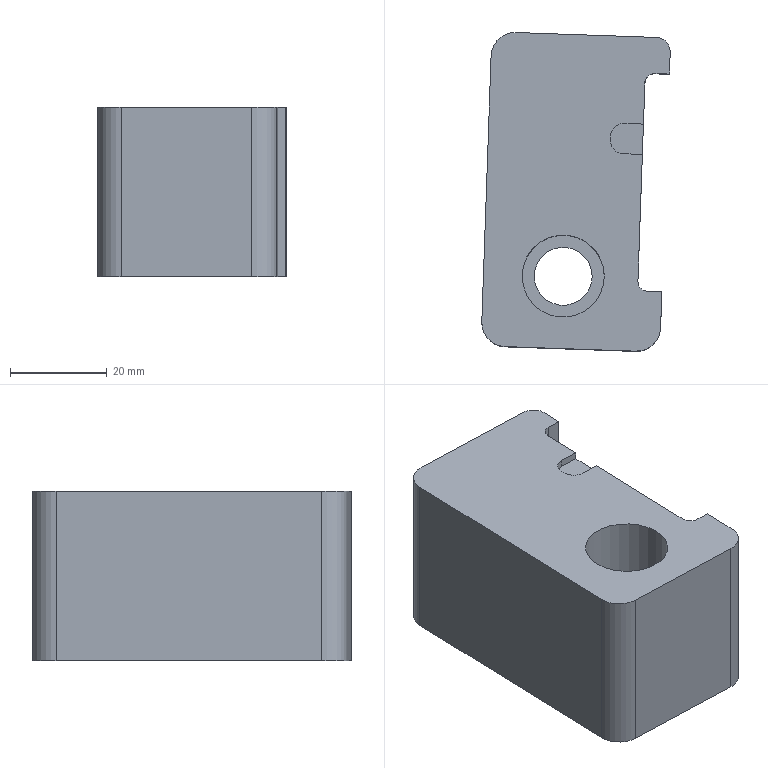Part | NX | features DIE-47 2 | 1 solid | 24 faces | box 38.971 x 65.909 x 35 mm | volume 68711 mm3 | plane 14 | cylinder 8 | spline 2 | commonest cylinder face diameters 10 x3 4.04 x2 6 x1 12.002 x1 17 x1
STEP:
#1=CARTESIAN_POINT('',(2946.663,-896.363,858.716));
#2=VERTEX_POINT('',#1);
#3=CARTESIAN_POINT('',(2946.371,-904.863,858.716));
#4=VERTEX_POINT('',#3);
#5=CARTESIAN_POINT('',(2945.852,-919.349,858.716));
#6=DIRECTION('',(0.0349,0.9994,0.));
#7=VECTOR('',#6,1000.);
#8=LINE('',#5,#7);
#9=EDGE_CURVE('',#2,#4,#8,.F.);
#10=ORIENTED_EDGE('',*,*,#9,.T.);
#11=CARTESIAN_POINT('',(2946.358,-904.862,857.216));
#12=VERTEX_POINT('',#11);
#13=CARTESIAN_POINT('',(2946.358,-904.862,858.716));
#14=DIRECTION('',(0.,0.,-1.));
#15=VECTOR('',#14,1000.);
#16=LINE('',#13,#15);
#17=EDGE_CURVE('',#4,#12,#16,.T.);
#18=ORIENTED_EDGE('',*,*,#17,.T.);
#19=CARTESIAN_POINT('',(2946.139,-911.133,857.216));
#20=VERTEX_POINT('',#19);
#21=CARTESIAN_POINT('',(2946.139,-911.133,857.216));
#22=CARTESIAN_POINT('',(2946.183,-909.878,857.216));
#23=CARTESIAN_POINT('',(2946.226,-908.624,857.216));
#24=CARTESIAN_POINT('',(2946.27,-907.37,857.216));
#25=CARTESIAN_POINT('',(2946.314,-906.116,857.216));
#26=CARTESIAN_POINT('',(2946.358,-904.862,857.216));
#27=B_SPLINE_CURVE_WITH_KNOTS('',5,(#21,#22,#23,#24,#25,#26),.UNSPECIFIED.,.F.,.F.,(6,6),(0.,1.),.PIECEWISE_BEZIER_KNOTS.);
#28=EDGE_CURVE('',#20,#12,#27,.T.);
#29=ORIENTED_EDGE('',*,*,#28,.F.);
#30=CARTESIAN_POINT('',(2946.139,-911.133,858.716));
#31=VERTEX_POINT('',#30);
#32=CARTESIAN_POINT('',(2946.139,-911.133,858.716));
#33=DIRECTION('',(0.,0.,-1.));
#34=VECTOR('',#33,1000.);
#35=LINE('',#32,#34);
#36=EDGE_CURVE('',#20,#31,#35,.F.);
#37=ORIENTED_EDGE('',*,*,#36,.T.);
#38=CARTESIAN_POINT('',(2945.224,-937.338,858.716));
#39=VERTEX_POINT('',#38);
#40=CARTESIAN_POINT('',(2945.852,-919.349,858.716));
#41=DIRECTION('',(0.0349,0.9994,0.));
#42=VECTOR('',#41,1000.);
#43=LINE('',#40,#42);
#44=EDGE_CURVE('',#31,#39,#43,.F.);
#45=ORIENTED_EDGE('',*,*,#44,.T.);
#46=CARTESIAN_POINT('',(2945.224,-937.338,823.716));
#47=VERTEX_POINT('',#46);
#48=CARTESIAN_POINT('',(2945.224,-937.338,858.716));
#49=DIRECTION('',(0.,0.,1.));
#50=VECTOR('',#49,1000.);
#51=LINE('',#48,#50);
#52=EDGE_CURVE('',#39,#47,#51,.F.);
#53=ORIENTED_EDGE('',*,*,#52,.T.);
#54=CARTESIAN_POINT('',(2946.655,-896.363,823.716));
#55=VERTEX_POINT('',#54);
#56=CARTESIAN_POINT('',(2945.852,-919.349,823.716));
#57=DIRECTION('',(0.0349,0.9994,0.));
#58=VECTOR('',#57,1000.);
#59=LINE('',#56,#58);
#60=EDGE_CURVE('',#47,#55,#59,.T.);
#61=ORIENTED_EDGE('',*,*,#60,.T.);
#62=CARTESIAN_POINT('',(2946.655,-896.363,858.716));
#63=DIRECTION('',(0.,0.,1.));
#64=VECTOR('',#63,1000.);
#65=LINE('',#62,#64);
#66=EDGE_CURVE('',#55,#2,#65,.T.);
#67=ORIENTED_EDGE('',*,*,#66,.T.);
#68=EDGE_LOOP('',(#10,#18,#29,#37,#45,#53,#61,#67));
#69=FACE_BOUND('',#68,.T.);
#70=CARTESIAN_POINT('',(2945.852,-919.349,858.716));
#71=DIRECTION('',(0.9994,-0.0349,0.));
#72=DIRECTION('',(0.0349,0.9994,0.));
#73=AXIS2_PLACEMENT_3D('',#70,#71,#72);
#74=PLANE('',#73);
#75=ADVANCED_FACE('',(#69),#74,.T.);
#76=CARTESIAN_POINT('',(2921.271,-936.298,858.716));
#77=VERTEX_POINT('',#76);
#78=CARTESIAN_POINT('',(2929.771,-936.298,858.716));
#79=DIRECTION('',(0.,0.,-1.));
#80=DIRECTION('',(-1.,0.,0.));
#81=AXIS2_PLACEMENT_3D('',#78,#79,#80);
#82=CIRCLE('',#81,8.5);
#83=EDGE_CURVE('',#77,#77,#82,.T.);
#84=ORIENTED_EDGE('',*,*,#83,.T.);
#85=EDGE_LOOP('',(#84));
#86=FACE_BOUND('',#85,.T.);
#87=CARTESIAN_POINT('',(2917.754,-950.887,858.716));
#88=VERTEX_POINT('',#87);
#89=CARTESIAN_POINT('',(2944.738,-951.829,858.716));
#90=VERTEX_POINT('',#89);
#91=CARTESIAN_POINT('',(2936.743,-951.55,858.716));
#92=DIRECTION('',(-0.9994,0.0349,0.));
#93=VECTOR('',#92,1000.);
#94=LINE('',#91,#93);
#95=EDGE_CURVE('',#88,#90,#94,.F.);
#96=ORIENTED_EDGE('',*,*,#95,.T.);
#97=CARTESIAN_POINT('',(2949.909,-947.007,858.716));
#98=VERTEX_POINT('',#97);
#99=CARTESIAN_POINT('',(2944.912,-946.833,858.716));
#100=DIRECTION('',(0.,0.,-1.));
#101=DIRECTION('',(-1.,0.,0.));
#102=AXIS2_PLACEMENT_3D('',#99,#100,#101);
#103=CIRCLE('',#102,5.);
#104=EDGE_CURVE('',#90,#98,#103,.F.);
#105=ORIENTED_EDGE('',*,*,#104,.T.);
#106=CARTESIAN_POINT('',(2950.17,-939.532,858.716));
#107=VERTEX_POINT('',#106);
#108=CARTESIAN_POINT('',(2950.869,-919.524,858.716));
#109=DIRECTION('',(0.0349,0.9994,0.));
#110=VECTOR('',#109,1000.);
#111=LINE('',#108,#110);
#112=EDGE_CURVE('',#107,#98,#111,.F.);
#113=ORIENTED_EDGE('',*,*,#112,.F.);
#114=CARTESIAN_POINT('',(2947.172,-939.427,858.716));
#115=VERTEX_POINT('',#114);
#116=CARTESIAN_POINT('',(2956.52,-939.753,858.716));
#117=DIRECTION('',(0.9994,-0.0349,0.));
#118=VECTOR('',#117,1000.);
#119=LINE('',#116,#118);
#120=EDGE_CURVE('',#107,#115,#119,.F.);
#121=ORIENTED_EDGE('',*,*,#120,.T.);
#122=CARTESIAN_POINT('',(2947.243,-937.408,858.716));
#123=DIRECTION('',(0.,0.,1.));
#124=DIRECTION('',(1.,0.,0.));
#125=AXIS2_PLACEMENT_3D('',#122,#123,#124);
#126=CIRCLE('',#125,2.02);
#127=EDGE_CURVE('',#39,#115,#126,.T.);
#128=ORIENTED_EDGE('',*,*,#127,.F.);
#129=ORIENTED_EDGE('',*,*,#44,.F.);
#130=CARTESIAN_POINT('',(2942.1,-910.991,858.716));
#131=VERTEX_POINT('',#130);
#132=CARTESIAN_POINT('',(2946.139,-911.133,858.716));
#133=CARTESIAN_POINT('',(2944.792,-911.086,858.716));
#134=CARTESIAN_POINT('',(2943.446,-911.039,858.716));
#135=CARTESIAN_POINT('',(2942.1,-910.991,858.716));
#136=B_SPLINE_CURVE_WITH_KNOTS('',3,(#132,#133,#134,#135),.UNSPECIFIED.,.F.,.F.,(4,4),(0.00502,0.009061),.UNSPECIFIED.);
#137=EDGE_CURVE('',#31,#131,#136,.T.);
#138=ORIENTED_EDGE('',*,*,#137,.T.);
#139=CARTESIAN_POINT('',(2940.946,-910.666,858.716));
#140=VERTEX_POINT('',#139);
#141=CARTESIAN_POINT('',(2942.1,-910.991,858.716));
#142=CARTESIAN_POINT('',(2941.681,-910.977,858.716));
#143=CARTESIAN_POINT('',(2941.297,-910.868,858.716));
#144=CARTESIAN_POINT('',(2940.946,-910.666,858.716));
#145=B_SPLINE_CURVE_WITH_KNOTS('',3,(#141,#142,#143,#144),.UNSPECIFIED.,.F.,.F.,(4,4),(0.,1.),.UNSPECIFIED.);
#146=EDGE_CURVE('',#131,#140,#145,.T.);
#147=ORIENTED_EDGE('',*,*,#146,.T.);
#148=CARTESIAN_POINT('',(2940.072,-909.843,858.716));
#149=VERTEX_POINT('',#148);
#150=CARTESIAN_POINT('',(2940.946,-910.666,858.716));
#151=CARTESIAN_POINT('',(2940.6,-910.467,858.716));
#152=CARTESIAN_POINT('',(2940.305,-910.184,858.716));
#153=CARTESIAN_POINT('',(2940.072,-909.843,858.716));
#154=B_SPLINE_CURVE_WITH_KNOTS('',3,(#150,#151,#152,#153),.UNSPECIFIED.,.F.,.F.,(4,4),(0.,1.),.UNSPECIFIED.);
#155=EDGE_CURVE('',#140,#149,#154,.T.);
#156=ORIENTED_EDGE('',*,*,#155,.T.);
#157=CARTESIAN_POINT('',(2939.671,-909.031,858.716));
#158=VERTEX_POINT('',#157);
#159=CARTESIAN_POINT('',(2940.072,-909.843,858.716));
#160=CARTESIAN_POINT('',(2939.904,-909.597,858.716));
#161=CARTESIAN_POINT('',(2939.77,-909.326,858.716));
#162=CARTESIAN_POINT('',(2939.671,-909.031,858.716));
#163=B_SPLINE_CURVE_WITH_KNOTS('',3,(#159,#160,#161,#162),.UNSPECIFIED.,.F.,.F.,(4,4),(0.,1.),.UNSPECIFIED.);
#164=EDGE_CURVE('',#149,#158,#163,.T.);
#165=ORIENTED_EDGE('',*,*,#164,.T.);
#166=CARTESIAN_POINT('',(2939.499,-907.537,858.716));
#167=VERTEX_POINT('',#166);
#168=CARTESIAN_POINT('',(2939.671,-909.031,858.716));
#169=CARTESIAN_POINT('',(2939.59,-908.79,858.716));
#170=CARTESIAN_POINT('',(2939.507,-908.413,858.716));
#171=CARTESIAN_POINT('',(2939.478,-907.989,858.716));
#172=CARTESIAN_POINT('',(2939.484,-907.712,858.716));
#173=CARTESIAN_POINT('',(2939.49,-907.634,858.716));
#174=CARTESIAN_POINT('',(2939.498,-907.537,858.716));
#175=B_SPLINE_CURVE_WITH_KNOTS('',3,(#168,#169,#170,#171,#172,#173,#174),.UNSPECIFIED.,.F.,.F.,(4,1,1,1,4),(0.,0.5,0.75,0.875,1.),.UNSPECIFIED.);
#176=EDGE_CURVE('',#158,#167,#175,.T.);
#177=ORIENTED_EDGE('',*,*,#176,.T.);
#178=CARTESIAN_POINT('',(2940.362,-905.554,858.716));
#179=VERTEX_POINT('',#178);
#180=CARTESIAN_POINT('',(2939.499,-907.537,858.716));
#181=CARTESIAN_POINT('',(2939.573,-906.799,858.716));
#182=CARTESIAN_POINT('',(2939.876,-906.079,858.716));
#183=CARTESIAN_POINT('',(2940.362,-905.554,858.716));
#184=B_SPLINE_CURVE_WITH_KNOTS('',3,(#180,#181,#182,#183),.UNSPECIFIED.,.F.,.F.,(4,4),(0.,1.),.UNSPECIFIED.);
#185=EDGE_CURVE('',#179,#167,#184,.F.);
#186=ORIENTED_EDGE('',*,*,#185,.F.);
#187=CARTESIAN_POINT('',(2941.247,-904.918,858.716));
#188=VERTEX_POINT('',#187);
#189=CARTESIAN_POINT('',(2940.362,-905.554,858.716));
#190=CARTESIAN_POINT('',(2940.616,-905.279,858.716));
#191=CARTESIAN_POINT('',(2940.914,-905.062,858.716));
#192=CARTESIAN_POINT('',(2941.247,-904.918,858.716));
#193=B_SPLINE_CURVE_WITH_KNOTS('',3,(#189,#190,#191,#192),.UNSPECIFIED.,.F.,.F.,(4,4),(0.,1.),.UNSPECIFIED.);
#194=EDGE_CURVE('',#188,#179,#193,.F.);
#195=ORIENTED_EDGE('',*,*,#194,.F.);
#196=CARTESIAN_POINT('',(2942.319,-904.721,858.716));
#197=VERTEX_POINT('',#196);
#198=CARTESIAN_POINT('',(2941.247,-904.918,858.716));
#199=CARTESIAN_POINT('',(2941.583,-904.774,858.716));
#200=CARTESIAN_POINT('',(2941.94,-904.708,858.716));
#201=CARTESIAN_POINT('',(2942.319,-904.721,858.716));
#202=B_SPLINE_CURVE_WITH_KNOTS('',3,(#198,#199,#200,#201),.UNSPECIFIED.,.F.,.F.,(4,4),(0.,1.),.UNSPECIFIED.);
#203=EDGE_CURVE('',#197,#188,#202,.F.);
#204=ORIENTED_EDGE('',*,*,#203,.F.);
#205=CARTESIAN_POINT('',(2942.319,-904.721,858.716));
#206=CARTESIAN_POINT('',(2943.674,-904.768,858.716));
#207=CARTESIAN_POINT('',(2945.029,-904.816,858.716));
#208=CARTESIAN_POINT('',(2946.384,-904.863,858.716));
#209=B_SPLINE_CURVE_WITH_KNOTS('',3,(#205,#206,#207,#208),.UNSPECIFIED.,.F.,.F.,(4,4),(0.,0.004068),.UNSPECIFIED.);
#210=EDGE_CURVE('',#197,#4,#209,.T.);
#211=ORIENTED_EDGE('',*,*,#210,.T.);
#212=ORIENTED_EDGE('',*,*,#9,.F.);
#213=CARTESIAN_POINT('',(2946.676,-896.134,858.716));
#214=VERTEX_POINT('',#213);
#215=CARTESIAN_POINT('',(2946.676,-896.134,858.716));
#216=CARTESIAN_POINT('',(2946.669,-896.21,858.716));
#217=CARTESIAN_POINT('',(2946.662,-896.286,858.716));
#218=CARTESIAN_POINT('',(2946.655,-896.363,858.716));
#219=B_SPLINE_CURVE_WITH_KNOTS('',3,(#215,#216,#217,#218),.UNSPECIFIED.,.F.,.F.,(4,4),(0.,1.),.UNSPECIFIED.);
#220=EDGE_CURVE('',#214,#2,#219,.T.);
#221=ORIENTED_EDGE('',*,*,#220,.F.);
#222=CARTESIAN_POINT('',(2948.744,-894.414,858.716));
#223=VERTEX_POINT('',#222);
#224=CARTESIAN_POINT('',(2948.673,-896.433,858.716));
#225=DIRECTION('',(0.,0.,1.));
#226=DIRECTION('',(1.,0.,0.));
#227=AXIS2_PLACEMENT_3D('',#224,#225,#226);
#228=CIRCLE('',#227,2.02);
#229=EDGE_CURVE('',#223,#214,#228,.T.);
#230=ORIENTED_EDGE('',*,*,#229,.F.);
#231=CARTESIAN_POINT('',(2951.742,-894.519,858.716));
#232=VERTEX_POINT('',#231);
#233=CARTESIAN_POINT('',(2958.092,-894.741,858.716));
#234=DIRECTION('',(0.9994,-0.0349,0.));
#235=VECTOR('',#234,1000.);
#236=LINE('',#233,#235);
#237=EDGE_CURVE('',#232,#223,#236,.F.);
#238=ORIENTED_EDGE('',*,*,#237,.F.);
#239=CARTESIAN_POINT('',(2951.898,-890.042,858.716));
#240=VERTEX_POINT('',#239);
#241=CARTESIAN_POINT('',(2950.869,-919.524,858.716));
#242=DIRECTION('',(0.0349,0.9994,0.));
#243=VECTOR('',#242,1000.);
#244=LINE('',#241,#243);
#245=EDGE_CURVE('',#240,#232,#244,.F.);
#246=ORIENTED_EDGE('',*,*,#245,.F.);
#247=CARTESIAN_POINT('',(2949.005,-886.939,858.716));
#248=VERTEX_POINT('',#247);
#249=CARTESIAN_POINT('',(2948.9,-889.937,858.716));
#250=DIRECTION('',(0.,0.,-1.));
#251=DIRECTION('',(-1.,0.,0.));
#252=AXIS2_PLACEMENT_3D('',#249,#250,#251);
#253=CIRCLE('',#252,3.);
#254=EDGE_CURVE('',#240,#248,#253,.F.);
#255=ORIENTED_EDGE('',*,*,#254,.T.);
#256=CARTESIAN_POINT('',(2920.022,-885.927,858.716));
#257=VERTEX_POINT('',#256);
#258=CARTESIAN_POINT('',(2939.011,-886.59,858.716));
#259=DIRECTION('',(-0.9994,0.0349,0.));
#260=VECTOR('',#259,1000.);
#261=LINE('',#258,#260);
#262=EDGE_CURVE('',#257,#248,#261,.F.);
#263=ORIENTED_EDGE('',*,*,#262,.F.);
#264=CARTESIAN_POINT('',(2914.851,-890.749,858.716));
#265=VERTEX_POINT('',#264);
#266=CARTESIAN_POINT('',(2919.848,-890.924,858.716));
#267=DIRECTION('',(0.,0.,-1.));
#268=DIRECTION('',(-1.,0.,0.));
#269=AXIS2_PLACEMENT_3D('',#266,#267,#268);
#270=CIRCLE('',#269,5.);
#271=EDGE_CURVE('',#257,#265,#270,.F.);
#272=ORIENTED_EDGE('',*,*,#271,.T.);
#273=CARTESIAN_POINT('',(2912.932,-945.716,858.716));
#274=VERTEX_POINT('',#273);
#275=CARTESIAN_POINT('',(2914.328,-905.74,858.716));
#276=DIRECTION('',(-0.0349,-0.9994,0.));
#277=VECTOR('',#276,1000.);
#278=LINE('',#275,#277);
#279=EDGE_CURVE('',#265,#274,#278,.T.);
#280=ORIENTED_EDGE('',*,*,#279,.T.);
#281=CARTESIAN_POINT('',(2917.929,-945.89,858.716));
#282=DIRECTION('',(0.,0.,-1.));
#283=DIRECTION('',(-1.,0.,0.));
#284=AXIS2_PLACEMENT_3D('',#281,#282,#283);
#285=CIRCLE('',#284,5.);
#286=EDGE_CURVE('',#274,#88,#285,.F.);
#287=ORIENTED_EDGE('',*,*,#286,.T.);
#288=EDGE_LOOP('',(#96,#105,#113,#121,#128,#129,#138,#147,#156,#165,#177,#186,#195,#204,#211,#212,#221,#230,#238,#246,#255,#263,#272,#280,#287));
#289=FACE_BOUND('',#288,.T.);
#290=CARTESIAN_POINT('',(2958.707,-877.122,858.716));
#291=DIRECTION('',(0.,0.,-1.));
#292=DIRECTION('',(0.,1.,0.));
#293=AXIS2_PLACEMENT_3D('',#290,#291,#292);
#294=PLANE('',#293);
#295=ADVANCED_FACE('',(#86,#289),#294,.F.);
#296=CARTESIAN_POINT('',(2951.742,-894.519,823.716));
#297=VERTEX_POINT('',#296);
#298=CARTESIAN_POINT('',(2951.742,-894.519,858.716));
#299=DIRECTION('',(0.,0.,1.));
#300=VECTOR('',#299,1000.);
#301=LINE('',#298,#300);
#302=EDGE_CURVE('',#232,#297,#301,.F.);
#303=ORIENTED_EDGE('',*,*,#302,.T.);
#304=CARTESIAN_POINT('',(2951.898,-890.042,823.716));
#305=VERTEX_POINT('',#304);
#306=CARTESIAN_POINT('',(2950.869,-919.524,823.716));
#307=DIRECTION('',(0.0349,0.9994,0.));
#308=VECTOR('',#307,1000.);
#309=LINE('',#306,#308);
#310=EDGE_CURVE('',#305,#297,#309,.F.);
#311=ORIENTED_EDGE('',*,*,#310,.F.);
#312=CARTESIAN_POINT('',(2951.898,-890.042,858.716));
#313=DIRECTION('',(0.,0.,1.));
#314=VECTOR('',#313,1000.);
#315=LINE('',#312,#314);
#316=EDGE_CURVE('',#305,#240,#315,.T.);
#317=ORIENTED_EDGE('',*,*,#316,.T.);
#318=ORIENTED_EDGE('',*,*,#245,.T.);
#319=EDGE_LOOP('',(#303,#311,#317,#318));
#320=FACE_BOUND('',#319,.T.);
#321=CARTESIAN_POINT('',(2950.869,-919.524,858.716));
#322=DIRECTION('',(0.9994,-0.0349,0.));
#323=DIRECTION('',(0.0349,0.9994,0.));
#324=AXIS2_PLACEMENT_3D('',#321,#322,#323);
#325=PLANE('',#324);
#326=ADVANCED_FACE('',(#320),#325,.T.);
#327=CARTESIAN_POINT('',(2917.754,-950.887,823.716));
#328=VERTEX_POINT('',#327);
#329=CARTESIAN_POINT('',(2912.932,-945.716,823.716));
#330=VERTEX_POINT('',#329);
#331=CARTESIAN_POINT('',(2917.929,-945.89,823.716));
#332=DIRECTION('',(0.,0.,-1.));
#333=DIRECTION('',(-1.,0.,0.));
#334=AXIS2_PLACEMENT_3D('',#331,#332,#333);
#335=CIRCLE('',#334,5.);
#336=EDGE_CURVE('',#328,#330,#335,.T.);
#337=ORIENTED_EDGE('',*,*,#336,.F.);
#338=CARTESIAN_POINT('',(2917.754,-950.887,935.716));
#339=DIRECTION('',(0.,0.,-1.));
#340=VECTOR('',#339,1000.);
#341=LINE('',#338,#340);
#342=EDGE_CURVE('',#88,#328,#341,.T.);
#343=ORIENTED_EDGE('',*,*,#342,.F.);
#344=ORIENTED_EDGE('',*,*,#286,.F.);
#345=CARTESIAN_POINT('',(2912.932,-945.716,898.213));
#346=DIRECTION('',(0.,0.,1.));
#347=VECTOR('',#346,1000.);
#348=LINE('',#345,#347);
#349=EDGE_CURVE('',#330,#274,#348,.T.);
#350=ORIENTED_EDGE('',*,*,#349,.F.);
#351=EDGE_LOOP('',(#337,#343,#344,#350));
#352=FACE_BOUND('',#351,.T.);
#353=CARTESIAN_POINT('',(2917.929,-945.89,935.716));
#354=DIRECTION('',(0.,0.,1.));
#355=DIRECTION('',(1.,0.,0.));
#356=AXIS2_PLACEMENT_3D('',#353,#354,#355);
#357=CYLINDRICAL_SURFACE('',#356,5.);
#358=ADVANCED_FACE('',(#352),#357,.T.);
#359=ORIENTED_EDGE('',*,*,#279,.F.);
#360=CARTESIAN_POINT('',(2914.851,-890.749,823.716));
#361=VERTEX_POINT('',#360);
#362=CARTESIAN_POINT('',(2914.851,-890.749,898.213));
#363=DIRECTION('',(0.,0.,1.));
#364=VECTOR('',#363,1000.);
#365=LINE('',#362,#364);
#366=EDGE_CURVE('',#265,#361,#365,.F.);
#367=ORIENTED_EDGE('',*,*,#366,.T.);
#368=CARTESIAN_POINT('',(2914.358,-904.859,823.716));
#369=DIRECTION('',(0.0349,0.9994,0.));
#370=VECTOR('',#369,1000.);
#371=LINE('',#368,#370);
#372=EDGE_CURVE('',#330,#361,#371,.T.);
#373=ORIENTED_EDGE('',*,*,#372,.F.);
#374=ORIENTED_EDGE('',*,*,#349,.T.);
#375=EDGE_LOOP('',(#359,#367,#373,#374));
#376=FACE_BOUND('',#375,.T.);
#377=CARTESIAN_POINT('',(2914.328,-905.74,898.213));
#378=DIRECTION('',(-0.9994,0.0349,0.));
#379=DIRECTION('',(-0.0349,-0.9994,0.));
#380=AXIS2_PLACEMENT_3D('',#377,#378,#379);
#381=PLANE('',#380);
#382=ADVANCED_FACE('',(#376),#381,.T.);
#383=CARTESIAN_POINT('',(2920.022,-885.927,823.716));
#384=VERTEX_POINT('',#383);
#385=CARTESIAN_POINT('',(2919.848,-890.924,823.716));
#386=DIRECTION('',(0.,0.,-1.));
#387=DIRECTION('',(-1.,0.,0.));
#388=AXIS2_PLACEMENT_3D('',#385,#386,#387);
#389=CIRCLE('',#388,5.);
#390=EDGE_CURVE('',#361,#384,#389,.T.);
#391=ORIENTED_EDGE('',*,*,#390,.F.);
#392=ORIENTED_EDGE('',*,*,#366,.F.);
#393=ORIENTED_EDGE('',*,*,#271,.F.);
#394=CARTESIAN_POINT('',(2920.022,-885.927,898.213));
#395=DIRECTION('',(0.,0.,-1.));
#396=VECTOR('',#395,1000.);
#397=LINE('',#394,#396);
#398=EDGE_CURVE('',#384,#257,#397,.F.);
#399=ORIENTED_EDGE('',*,*,#398,.F.);
#400=EDGE_LOOP('',(#391,#392,#393,#399));
#401=FACE_BOUND('',#400,.T.);
#402=CARTESIAN_POINT('',(2919.848,-890.924,898.213));
#403=DIRECTION('',(0.,0.,-1.));
#404=DIRECTION('',(-1.,0.,0.));
#405=AXIS2_PLACEMENT_3D('',#402,#403,#404);
#406=CYLINDRICAL_SURFACE('',#405,5.);
#407=ADVANCED_FACE('',(#401),#406,.T.);
#408=CARTESIAN_POINT('',(2944.738,-951.829,823.716));
#409=VERTEX_POINT('',#408);
#410=CARTESIAN_POINT('',(2965.665,-952.56,823.716));
#411=DIRECTION('',(0.9994,-0.0349,0.));
#412=VECTOR('',#411,1000.);
#413=LINE('',#410,#412);
#414=EDGE_CURVE('',#409,#328,#413,.F.);
#415=ORIENTED_EDGE('',*,*,#414,.F.);
#416=CARTESIAN_POINT('',(2944.738,-951.829,935.716));
#417=DIRECTION('',(0.,0.,1.));
#418=VECTOR('',#417,1000.);
#419=LINE('',#416,#418);
#420=EDGE_CURVE('',#409,#90,#419,.T.);
#421=ORIENTED_EDGE('',*,*,#420,.T.);
#422=ORIENTED_EDGE('',*,*,#95,.F.);
#423=ORIENTED_EDGE('',*,*,#342,.T.);
#424=EDGE_LOOP('',(#415,#421,#422,#423));
#425=FACE_BOUND('',#424,.T.);
#426=CARTESIAN_POINT('',(2936.743,-951.55,935.716));
#427=DIRECTION('',(0.0349,0.9994,0.));
#428=DIRECTION('',(-0.9994,0.0349,0.));
#429=AXIS2_PLACEMENT_3D('',#426,#427,#428);
#430=PLANE('',#429);
#431=ADVANCED_FACE('',(#425),#430,.F.);
#432=ORIENTED_EDGE('',*,*,#262,.T.);
#433=CARTESIAN_POINT('',(2949.005,-886.939,823.716));
#434=VERTEX_POINT('',#433);
#435=CARTESIAN_POINT('',(2949.005,-886.939,823.716));
#436=DIRECTION('',(0.,0.,-1.));
#437=VECTOR('',#436,1000.);
#438=LINE('',#435,#437);
#439=EDGE_CURVE('',#248,#434,#438,.T.);
#440=ORIENTED_EDGE('',*,*,#439,.T.);
#441=CARTESIAN_POINT('',(2967.933,-887.6,823.716));
#442=DIRECTION('',(0.9994,-0.0349,0.));
#443=VECTOR('',#442,1000.);
#444=LINE('',#441,#443);
#445=EDGE_CURVE('',#434,#384,#444,.F.);
#446=ORIENTED_EDGE('',*,*,#445,.T.);
#447=ORIENTED_EDGE('',*,*,#398,.T.);
#448=EDGE_LOOP('',(#432,#440,#446,#447));
#449=FACE_BOUND('',#448,.T.);
#450=CARTESIAN_POINT('',(2939.011,-886.59,935.716));
#451=DIRECTION('',(0.0349,0.9994,0.));
#452=DIRECTION('',(-0.9994,0.0349,0.));
#453=AXIS2_PLACEMENT_3D('',#450,#451,#452);
#454=PLANE('',#453);
#455=ADVANCED_FACE('',(#449),#454,.T.);
#456=CARTESIAN_POINT('',(2923.77,-936.298,823.716));
#457=VERTEX_POINT('',#456);
#458=CARTESIAN_POINT('',(2929.771,-936.298,823.716));
#459=DIRECTION('',(0.,0.,-1.));
#460=DIRECTION('',(-1.,0.,0.));
#461=AXIS2_PLACEMENT_3D('',#458,#459,#460);
#462=CIRCLE('',#461,6.001);
#463=EDGE_CURVE('',#457,#457,#462,.T.);
#464=ORIENTED_EDGE('',*,*,#463,.F.);
#465=EDGE_LOOP('',(#464));
#466=FACE_BOUND('',#465,.T.);
#467=CARTESIAN_POINT('',(2950.17,-939.532,823.716));
#468=VERTEX_POINT('',#467);
#469=CARTESIAN_POINT('',(2949.909,-947.007,823.716));
#470=VERTEX_POINT('',#469);
#471=CARTESIAN_POINT('',(2950.869,-919.524,823.716));
#472=DIRECTION('',(0.0349,0.9994,0.));
#473=VECTOR('',#472,1000.);
#474=LINE('',#471,#473);
#475=EDGE_CURVE('',#468,#470,#474,.F.);
#476=ORIENTED_EDGE('',*,*,#475,.T.);
#477=CARTESIAN_POINT('',(2944.912,-946.833,823.716));
#478=DIRECTION('',(0.,0.,-1.));
#479=DIRECTION('',(-1.,0.,0.));
#480=AXIS2_PLACEMENT_3D('',#477,#478,#479);
#481=CIRCLE('',#480,5.);
#482=EDGE_CURVE('',#470,#409,#481,.T.);
#483=ORIENTED_EDGE('',*,*,#482,.T.);
#484=ORIENTED_EDGE('',*,*,#414,.T.);
#485=ORIENTED_EDGE('',*,*,#336,.T.);
#486=ORIENTED_EDGE('',*,*,#372,.T.);
#487=ORIENTED_EDGE('',*,*,#390,.T.);
#488=ORIENTED_EDGE('',*,*,#445,.F.);
#489=CARTESIAN_POINT('',(2948.9,-889.937,823.716));
#490=DIRECTION('',(0.,0.,-1.));
#491=DIRECTION('',(-1.,0.,0.));
#492=AXIS2_PLACEMENT_3D('',#489,#490,#491);
#493=CIRCLE('',#492,3.);
#494=EDGE_CURVE('',#434,#305,#493,.T.);
#495=ORIENTED_EDGE('',*,*,#494,.T.);
#496=ORIENTED_EDGE('',*,*,#310,.T.);
#497=CARTESIAN_POINT('',(2948.744,-894.414,823.716));
#498=VERTEX_POINT('',#497);
#499=CARTESIAN_POINT('',(2967.672,-895.075,823.716));
#500=DIRECTION('',(0.9994,-0.0349,0.));
#501=VECTOR('',#500,1000.);
#502=LINE('',#499,#501);
#503=EDGE_CURVE('',#297,#498,#502,.F.);
#504=ORIENTED_EDGE('',*,*,#503,.T.);
#505=CARTESIAN_POINT('',(2948.673,-896.433,823.716));
#506=DIRECTION('',(0.,0.,1.));
#507=DIRECTION('',(1.,0.,0.));
#508=AXIS2_PLACEMENT_3D('',#505,#506,#507);
#509=CIRCLE('',#508,2.02);
#510=EDGE_CURVE('',#55,#498,#509,.F.);
#511=ORIENTED_EDGE('',*,*,#510,.F.);
#512=ORIENTED_EDGE('',*,*,#60,.F.);
#513=CARTESIAN_POINT('',(2947.172,-939.427,823.716));
#514=VERTEX_POINT('',#513);
#515=CARTESIAN_POINT('',(2947.243,-937.408,823.716));
#516=DIRECTION('',(0.,0.,1.));
#517=DIRECTION('',(1.,0.,0.));
#518=AXIS2_PLACEMENT_3D('',#515,#516,#517);
#519=CIRCLE('',#518,2.02);
#520=EDGE_CURVE('',#47,#514,#519,.T.);
#521=ORIENTED_EDGE('',*,*,#520,.T.);
#522=CARTESIAN_POINT('',(2966.1,-940.088,823.716));
#523=DIRECTION('',(0.9994,-0.0349,0.));
#524=VECTOR('',#523,1000.);
#525=LINE('',#522,#524);
#526=EDGE_CURVE('',#514,#468,#525,.T.);
#527=ORIENTED_EDGE('',*,*,#526,.T.);
#528=EDGE_LOOP('',(#476,#483,#484,#485,#486,#487,#488,#495,#496,#504,#511,#512,#521,#527));
#529=FACE_BOUND('',#528,.T.);
#530=CARTESIAN_POINT('',(2967.266,-906.707,823.716));
#531=DIRECTION('',(0.,0.,-1.));
#532=DIRECTION('',(0.0349,0.9994,0.));
#533=AXIS2_PLACEMENT_3D('',#530,#531,#532);
#534=PLANE('',#533);
#535=ADVANCED_FACE('',(#466,#529),#534,.T.);
#536=ORIENTED_EDGE('',*,*,#112,.T.);
#537=CARTESIAN_POINT('',(2949.909,-947.007,858.716));
#538=DIRECTION('',(0.,0.,-1.));
#539=VECTOR('',#538,1000.);
#540=LINE('',#537,#539);
#541=EDGE_CURVE('',#98,#470,#540,.T.);
#542=ORIENTED_EDGE('',*,*,#541,.T.);
#543=ORIENTED_EDGE('',*,*,#475,.F.);
#544=CARTESIAN_POINT('',(2950.17,-939.532,858.716));
#545=DIRECTION('',(0.,0.,1.));
#546=VECTOR('',#545,1000.);
#547=LINE('',#544,#546);
#548=EDGE_CURVE('',#468,#107,#547,.T.);
#549=ORIENTED_EDGE('',*,*,#548,.T.);
#550=EDGE_LOOP('',(#536,#542,#543,#549));
#551=FACE_BOUND('',#550,.T.);
#552=CARTESIAN_POINT('',(2950.869,-919.524,858.716));
#553=DIRECTION('',(0.9994,-0.0349,0.));
#554=DIRECTION('',(0.0349,0.9994,0.));
#555=AXIS2_PLACEMENT_3D('',#552,#553,#554);
#556=PLANE('',#555);
#557=ADVANCED_FACE('',(#551),#556,.T.);
#558=ORIENTED_EDGE('',*,*,#254,.F.);
#559=ORIENTED_EDGE('',*,*,#316,.F.);
#560=ORIENTED_EDGE('',*,*,#494,.F.);
#561=ORIENTED_EDGE('',*,*,#439,.F.);
#562=EDGE_LOOP('',(#558,#559,#560,#561));
#563=FACE_BOUND('',#562,.T.);
#564=CARTESIAN_POINT('',(2948.9,-889.937,935.716));
#565=DIRECTION('',(0.,0.,-1.));
#566=DIRECTION('',(-1.,0.,0.));
#567=AXIS2_PLACEMENT_3D('',#564,#565,#566);
#568=CYLINDRICAL_SURFACE('',#567,3.);
#569=ADVANCED_FACE('',(#563),#568,.T.);
#570=ORIENTED_EDGE('',*,*,#237,.T.);
#571=CARTESIAN_POINT('',(2948.744,-894.414,858.716));
#572=DIRECTION('',(0.,0.,1.));
#573=VECTOR('',#572,1000.);
#574=LINE('',#571,#573);
#575=EDGE_CURVE('',#223,#498,#574,.F.);
#576=ORIENTED_EDGE('',*,*,#575,.T.);
#577=ORIENTED_EDGE('',*,*,#503,.F.);
#578=ORIENTED_EDGE('',*,*,#302,.F.);
#579=EDGE_LOOP('',(#570,#576,#577,#578));
#580=FACE_BOUND('',#579,.T.);
#581=CARTESIAN_POINT('',(2938.75,-894.065,935.716));
#582=DIRECTION('',(0.0349,0.9994,0.));
#583=DIRECTION('',(-0.9994,0.0349,0.));
#584=AXIS2_PLACEMENT_3D('',#581,#582,#583);
#585=PLANE('',#584);
#586=ADVANCED_FACE('',(#580),#585,.F.);
#587=ORIENTED_EDGE('',*,*,#220,.T.);
#588=ORIENTED_EDGE('',*,*,#66,.F.);
#589=ORIENTED_EDGE('',*,*,#510,.T.);
#590=ORIENTED_EDGE('',*,*,#575,.F.);
#591=ORIENTED_EDGE('',*,*,#229,.T.);
#592=EDGE_LOOP('',(#587,#588,#589,#590,#591));
#593=FACE_BOUND('',#592,.T.);
#594=CARTESIAN_POINT('',(2948.673,-896.433,858.716));
#595=DIRECTION('',(0.,0.,1.));
#596=DIRECTION('',(1.,0.,0.));
#597=AXIS2_PLACEMENT_3D('',#594,#595,#596);
#598=CYLINDRICAL_SURFACE('',#597,2.02);
#599=ADVANCED_FACE('',(#593),#598,.F.);
#600=CARTESIAN_POINT('',(2947.172,-939.427,858.716));
#601=DIRECTION('',(0.,0.,1.));
#602=VECTOR('',#601,1000.);
#603=LINE('',#600,#602);
#604=EDGE_CURVE('',#514,#115,#603,.T.);
#605=ORIENTED_EDGE('',*,*,#604,.F.);
#606=ORIENTED_EDGE('',*,*,#520,.F.);
#607=ORIENTED_EDGE('',*,*,#52,.F.);
#608=ORIENTED_EDGE('',*,*,#127,.T.);
#609=EDGE_LOOP('',(#605,#606,#607,#608));
#610=FACE_BOUND('',#609,.T.);
#611=CARTESIAN_POINT('',(2947.243,-937.408,858.716));
#612=DIRECTION('',(0.,0.,1.));
#613=DIRECTION('',(1.,0.,0.));
#614=AXIS2_PLACEMENT_3D('',#611,#612,#613);
#615=CYLINDRICAL_SURFACE('',#614,2.02);
#616=ADVANCED_FACE('',(#610),#615,.F.);
#617=ORIENTED_EDGE('',*,*,#548,.F.);
#618=ORIENTED_EDGE('',*,*,#526,.F.);
#619=ORIENTED_EDGE('',*,*,#604,.T.);
#620=ORIENTED_EDGE('',*,*,#120,.F.);
#621=EDGE_LOOP('',(#617,#618,#619,#620));
#622=FACE_BOUND('',#621,.T.);
#623=CARTESIAN_POINT('',(2937.178,-939.078,935.716));
#624=DIRECTION('',(0.0349,0.9994,0.));
#625=DIRECTION('',(-0.9994,0.0349,0.));
#626=AXIS2_PLACEMENT_3D('',#623,#624,#625);
#627=PLANE('',#626);
#628=ADVANCED_FACE('',(#622),#627,.T.);
#629=CARTESIAN_POINT('',(2921.271,-936.298,832.716));
#630=VERTEX_POINT('',#629);
#631=CARTESIAN_POINT('',(2929.771,-936.298,832.716));
#632=DIRECTION('',(0.,0.,-1.));
#633=DIRECTION('',(-1.,0.,0.));
#634=AXIS2_PLACEMENT_3D('',#631,#632,#633);
#635=CIRCLE('',#634,8.5);
#636=EDGE_CURVE('',#630,#630,#635,.T.);
#637=ORIENTED_EDGE('',*,*,#636,.T.);
#638=EDGE_LOOP('',(#637));
#639=FACE_BOUND('',#638,.T.);
#640=ORIENTED_EDGE('',*,*,#83,.F.);
#641=EDGE_LOOP('',(#640));
#642=FACE_BOUND('',#641,.T.);
#643=CARTESIAN_POINT('',(2929.771,-936.298,843.716));
#644=DIRECTION('',(0.,0.,1.));
#645=DIRECTION('',(1.,0.,0.));
#646=AXIS2_PLACEMENT_3D('',#643,#644,#645);
#647=CYLINDRICAL_SURFACE('',#646,8.5);
#648=ADVANCED_FACE('',(#639,#642),#647,.F.);
#649=ORIENTED_EDGE('',*,*,#463,.T.);
#650=EDGE_LOOP('',(#649));
#651=FACE_BOUND('',#650,.T.);
#652=CARTESIAN_POINT('',(2923.77,-936.298,832.716));
#653=VERTEX_POINT('',#652);
#654=CARTESIAN_POINT('',(2929.771,-936.298,832.716));
#655=DIRECTION('',(0.,0.,-1.));
#656=DIRECTION('',(-1.,0.,0.));
#657=AXIS2_PLACEMENT_3D('',#654,#655,#656);
#658=CIRCLE('',#657,6.001);
#659=EDGE_CURVE('',#653,#653,#658,.T.);
#660=ORIENTED_EDGE('',*,*,#659,.F.);
#661=EDGE_LOOP('',(#660));
#662=FACE_BOUND('',#661,.T.);
#663=CARTESIAN_POINT('',(2929.771,-936.298,808.716));
#664=DIRECTION('',(0.,0.,1.));
#665=DIRECTION('',(1.,0.,0.));
#666=AXIS2_PLACEMENT_3D('',#663,#664,#665);
#667=CYLINDRICAL_SURFACE('',#666,6.001);
#668=ADVANCED_FACE('',(#651,#662),#667,.F.);
#669=ORIENTED_EDGE('',*,*,#659,.T.);
#670=EDGE_LOOP('',(#669));
#671=FACE_BOUND('',#670,.T.);
#672=ORIENTED_EDGE('',*,*,#636,.F.);
#673=EDGE_LOOP('',(#672));
#674=FACE_BOUND('',#673,.T.);
#675=CARTESIAN_POINT('',(2929.771,-936.298,832.716));
#676=DIRECTION('',(0.,0.,-1.));
#677=DIRECTION('',(-1.,0.,0.));
#678=AXIS2_PLACEMENT_3D('',#675,#676,#677);
#679=PLANE('',#678);
#680=ADVANCED_FACE('',(#671,#674),#679,.F.);
#681=ORIENTED_EDGE('',*,*,#482,.F.);
#682=ORIENTED_EDGE('',*,*,#541,.F.);
#683=ORIENTED_EDGE('',*,*,#104,.F.);
#684=ORIENTED_EDGE('',*,*,#420,.F.);
#685=EDGE_LOOP('',(#681,#682,#683,#684));
#686=FACE_BOUND('',#685,.T.);
#687=CARTESIAN_POINT('',(2944.912,-946.833,935.716));
#688=DIRECTION('',(0.,0.,-1.));
#689=DIRECTION('',(-1.,0.,0.));
#690=AXIS2_PLACEMENT_3D('',#687,#688,#689);
#691=CYLINDRICAL_SURFACE('',#690,5.);
#692=ADVANCED_FACE('',(#686),#691,.T.);
#693=ORIENTED_EDGE('',*,*,#28,.T.);
#694=CARTESIAN_POINT('',(2942.319,-904.721,857.216));
#695=VERTEX_POINT('',#694);
#696=CARTESIAN_POINT('',(2942.319,-904.721,857.216));
#697=CARTESIAN_POINT('',(2942.493,-904.727,857.216));
#698=CARTESIAN_POINT('',(2942.668,-904.733,857.216));
#699=CARTESIAN_POINT('',(2942.843,-904.739,857.216));
#700=CARTESIAN_POINT('',(2943.842,-904.774,857.216));
#701=CARTESIAN_POINT('',(2944.841,-904.809,857.216));
#702=CARTESIAN_POINT('',(2945.841,-904.844,857.216));
#703=CARTESIAN_POINT('',(2946.022,-904.85,857.216));
#704=CARTESIAN_POINT('',(2946.203,-904.857,857.216));
#705=CARTESIAN_POINT('',(2946.384,-904.863,857.216));
#706=B_SPLINE_CURVE_WITH_KNOTS('',3,(#696,#697,#698,#699,#700,#701,#702,#703,#704,#705),.UNSPECIFIED.,.F.,.F.,(4,3,3,4),(0.,0.1289,0.8664,1.),.PIECEWISE_BEZIER_KNOTS.);
#707=EDGE_CURVE('',#695,#12,#706,.T.);
#708=ORIENTED_EDGE('',*,*,#707,.F.);
#709=CARTESIAN_POINT('',(2939.499,-907.537,857.216));
#710=VERTEX_POINT('',#709);
#711=CARTESIAN_POINT('',(2939.499,-907.537,857.216));
#712=CARTESIAN_POINT('',(2939.573,-906.803,857.216));
#713=CARTESIAN_POINT('',(2939.866,-906.09,857.216));
#714=CARTESIAN_POINT('',(2940.61,-905.285,857.216));
#715=CARTESIAN_POINT('',(2940.912,-905.063,857.216));
#716=CARTESIAN_POINT('',(2941.583,-904.774,857.216));
#717=CARTESIAN_POINT('',(2941.95,-904.708,857.216));
#718=CARTESIAN_POINT('',(2942.319,-904.721,857.216));
#719=B_SPLINE_CURVE_WITH_KNOTS('',3,(#711,#712,#713,#714,#715,#716,#717,#718),.UNSPECIFIED.,.F.,.F.,(4,2,2,4),(0.,0.5,0.75,1.),.UNSPECIFIED.);
#720=EDGE_CURVE('',#710,#695,#719,.T.);
#721=ORIENTED_EDGE('',*,*,#720,.F.);
#722=CARTESIAN_POINT('',(2942.1,-910.991,857.216));
#723=VERTEX_POINT('',#722);
#724=CARTESIAN_POINT('',(2942.1,-910.991,857.216));
#725=CARTESIAN_POINT('',(2941.693,-910.977,857.216));
#726=CARTESIAN_POINT('',(2941.294,-910.867,857.216));
#727=CARTESIAN_POINT('',(2940.598,-910.465,857.216));
#728=CARTESIAN_POINT('',(2940.3,-910.177,857.216));
#729=CARTESIAN_POINT('',(2939.843,-909.508,857.216));
#730=CARTESIAN_POINT('',(2939.682,-909.131,857.216));
#731=CARTESIAN_POINT('',(2939.489,-908.345,857.216));
#732=CARTESIAN_POINT('',(2939.464,-907.942,857.216));
#733=CARTESIAN_POINT('',(2939.498,-907.537,857.216));
#734=B_SPLINE_CURVE_WITH_KNOTS('',3,(#724,#725,#726,#727,#728,#729,#730,#731,#732,#733),.UNSPECIFIED.,.F.,.F.,(4,2,2,2,4),(0.,0.25,0.5,0.75,1.),.UNSPECIFIED.);
#735=EDGE_CURVE('',#723,#710,#734,.T.);
#736=ORIENTED_EDGE('',*,*,#735,.F.);
#737=CARTESIAN_POINT('',(2946.139,-911.133,857.216));
#738=CARTESIAN_POINT('',(2944.792,-911.086,857.216));
#739=CARTESIAN_POINT('',(2943.446,-911.039,857.216));
#740=CARTESIAN_POINT('',(2942.1,-910.991,857.216));
#741=B_SPLINE_CURVE_WITH_KNOTS('',3,(#737,#738,#739,#740),.UNSPECIFIED.,.F.,.F.,(4,4),(0.,1.),.PIECEWISE_BEZIER_KNOTS.);
#742=EDGE_CURVE('',#20,#723,#741,.T.);
#743=ORIENTED_EDGE('',*,*,#742,.F.);
#744=EDGE_LOOP('',(#693,#708,#721,#736,#743));
#745=FACE_BOUND('',#744,.T.);
#746=CARTESIAN_POINT('',(2939.498,-907.537,857.216));
#747=DIRECTION('',(0.,0.,1.));
#748=DIRECTION('',(0.,-1.,0.));
#749=AXIS2_PLACEMENT_3D('',#746,#747,#748);
#750=PLANE('',#749);
#751=ADVANCED_FACE('',(#745),#750,.T.);
#752=ORIENTED_EDGE('',*,*,#720,.T.);
#753=CARTESIAN_POINT('',(2942.319,-904.721,858.716));
#754=DIRECTION('',(0.,0.,-1.));
#755=VECTOR('',#754,1000.);
#756=LINE('',#753,#755);
#757=EDGE_CURVE('',#197,#695,#756,.T.);
#758=ORIENTED_EDGE('',*,*,#757,.F.);
#759=ORIENTED_EDGE('',*,*,#203,.T.);
#760=ORIENTED_EDGE('',*,*,#194,.T.);
#761=ORIENTED_EDGE('',*,*,#185,.T.);
#762=CARTESIAN_POINT('',(2939.499,-907.537,857.216));
#763=CARTESIAN_POINT('',(2939.499,-907.537,857.716));
#764=CARTESIAN_POINT('',(2939.499,-907.537,858.216));
#765=CARTESIAN_POINT('',(2939.499,-907.537,858.716));
#766=B_SPLINE_CURVE_WITH_KNOTS('',3,(#762,#763,#764,#765),.UNSPECIFIED.,.F.,.F.,(4,4),(0.,1.),.UNSPECIFIED.);
#767=EDGE_CURVE('',#167,#710,#766,.F.);
#768=ORIENTED_EDGE('',*,*,#767,.T.);
#769=EDGE_LOOP('',(#752,#758,#759,#760,#761,#768));
#770=FACE_BOUND('',#769,.T.);
#771=CARTESIAN_POINT('',(2939.499,-907.537,858.716));
#772=CARTESIAN_POINT('',(2939.499,-907.537,857.216));
#773=CARTESIAN_POINT('',(2939.573,-906.803,858.716));
#774=CARTESIAN_POINT('',(2939.573,-906.803,857.216));
#775=CARTESIAN_POINT('',(2940.147,-905.358,858.716));
#776=CARTESIAN_POINT('',(2940.147,-905.358,857.216));
#777=CARTESIAN_POINT('',(2941.581,-904.695,858.716));
#778=CARTESIAN_POINT('',(2941.581,-904.695,857.216));
#779=CARTESIAN_POINT('',(2942.319,-904.721,858.716));
#780=CARTESIAN_POINT('',(2942.319,-904.721,857.216));
#781=B_SPLINE_SURFACE_WITH_KNOTS('',3,1,((#771,#772),(#773,#774),(#775,#776),(#777,#778),(#779,#780)),.SURF_OF_LINEAR_EXTRUSION.,.F.,.F.,.F.,(4,1,4),(2,2),(0.,0.5,1.),(0.,1.),.UNSPECIFIED.);
#782=ADVANCED_FACE('',(#770),#781,.F.);
#783=ORIENTED_EDGE('',*,*,#735,.T.);
#784=ORIENTED_EDGE('',*,*,#767,.F.);
#785=ORIENTED_EDGE('',*,*,#176,.F.);
#786=ORIENTED_EDGE('',*,*,#164,.F.);
#787=ORIENTED_EDGE('',*,*,#155,.F.);
#788=ORIENTED_EDGE('',*,*,#146,.F.);
#789=CARTESIAN_POINT('',(2942.1,-910.991,858.716));
#790=CARTESIAN_POINT('',(2942.1,-910.991,858.216));
#791=CARTESIAN_POINT('',(2942.1,-910.991,857.716));
#792=CARTESIAN_POINT('',(2942.1,-910.991,857.216));
#793=B_SPLINE_CURVE_WITH_KNOTS('',3,(#789,#790,#791,#792),.UNSPECIFIED.,.F.,.F.,(4,4),(0.,1.),.UNSPECIFIED.);
#794=EDGE_CURVE('',#131,#723,#793,.T.);
#795=ORIENTED_EDGE('',*,*,#794,.T.);
#796=EDGE_LOOP('',(#783,#784,#785,#786,#787,#788,#795));
#797=FACE_BOUND('',#796,.T.);
#798=CARTESIAN_POINT('',(2942.1,-910.991,858.716));
#799=CARTESIAN_POINT('',(2942.1,-910.991,857.216));
#800=CARTESIAN_POINT('',(2941.286,-910.963,858.716));
#801=CARTESIAN_POINT('',(2941.286,-910.963,857.216));
#802=CARTESIAN_POINT('',(2939.786,-910.03,858.716));
#803=CARTESIAN_POINT('',(2939.786,-910.03,857.216));
#804=CARTESIAN_POINT('',(2939.429,-908.347,858.716));
#805=CARTESIAN_POINT('',(2939.429,-908.347,857.216));
#806=CARTESIAN_POINT('',(2939.498,-907.537,858.716));
#807=CARTESIAN_POINT('',(2939.498,-907.537,857.216));
#808=B_SPLINE_SURFACE_WITH_KNOTS('',3,1,((#798,#799),(#800,#801),(#802,#803),(#804,#805),(#806,#807)),.SURF_OF_LINEAR_EXTRUSION.,.F.,.F.,.F.,(4,1,4),(2,2),(0.,0.5,1.),(0.,1.),.UNSPECIFIED.);
#809=ADVANCED_FACE('',(#797),#808,.F.);
#810=ORIENTED_EDGE('',*,*,#742,.T.);
#811=ORIENTED_EDGE('',*,*,#794,.F.);
#812=ORIENTED_EDGE('',*,*,#137,.F.);
#813=ORIENTED_EDGE('',*,*,#36,.F.);
#814=EDGE_LOOP('',(#810,#811,#812,#813));
#815=FACE_BOUND('',#814,.T.);
#816=CARTESIAN_POINT('',(2946.139,-911.133,858.716));
#817=DIRECTION('',(-0.0349,-0.9994,0.));
#818=DIRECTION('',(0.9994,-0.0349,0.));
#819=AXIS2_PLACEMENT_3D('',#816,#817,#818);
#820=PLANE('',#819);
#821=ADVANCED_FACE('',(#815),#820,.F.);
#822=ORIENTED_EDGE('',*,*,#17,.F.);
#823=ORIENTED_EDGE('',*,*,#210,.F.);
#824=ORIENTED_EDGE('',*,*,#757,.T.);
#825=ORIENTED_EDGE('',*,*,#707,.T.);
#826=EDGE_LOOP('',(#822,#823,#824,#825));
#827=FACE_BOUND('',#826,.T.);
#828=CARTESIAN_POINT('',(2942.319,-904.721,858.716));
#829=DIRECTION('',(0.0349,0.9994,0.));
#830=DIRECTION('',(-0.9994,0.0349,0.));
#831=AXIS2_PLACEMENT_3D('',#828,#829,#830);
#832=PLANE('',#831);
#833=ADVANCED_FACE('',(#827),#832,.F.);
#834=CLOSED_SHELL('',(#75,#295,#326,#358,#382,#407,#431,#455,#535,#557,#569,#586,#599,#616,#628,#648,#668,#680,#692,#751,#782,#809,#821,#833));
#835=MANIFOLD_SOLID_BREP('',#834);
#836=(LENGTH_UNIT()NAMED_UNIT(*)SI_UNIT(.MILLI.,.METRE.));
#837=UNCERTAINTY_MEASURE_WITH_UNIT(LENGTH_MEASURE(0.06944),#836,'','');
#838=(NAMED_UNIT(*)PLANE_ANGLE_UNIT()SI_UNIT($,.RADIAN.));
#839=(NAMED_UNIT(*)SI_UNIT($,.STERADIAN.)SOLID_ANGLE_UNIT());
#840=(GEOMETRIC_REPRESENTATION_CONTEXT(3)GLOBAL_UNCERTAINTY_ASSIGNED_CONTEXT((#837))GLOBAL_UNIT_ASSIGNED_CONTEXT((#836,#838,#839))REPRESENTATION_CONTEXT('',''));
#841=ADVANCED_BREP_SHAPE_REPRESENTATION('',(#835),#840);